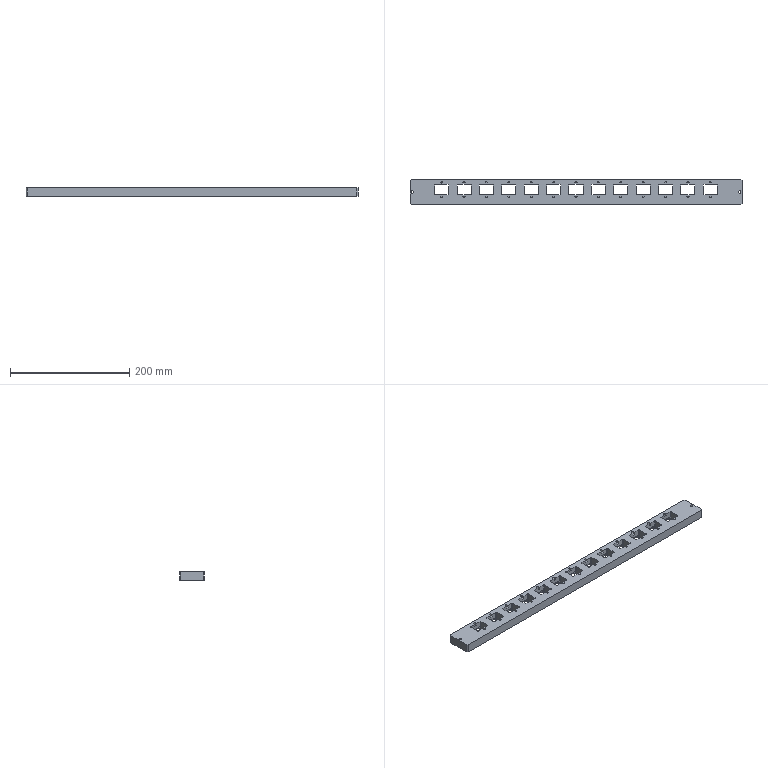NC program | NX | posted with a generic post | part box 556 x 41 x 15 mm
Lines 1 to 1304 of 144595:
N10 G17 G21 G94 G90
(ZLEVEL_PROFILE , TOOL : D10C)
N12 T10 M6
N14 G54
N16 G17 G0 G90 X-283.1 Y-3.442 S3500 M3
N18 G43 Z30. H10
N20 Z1.5
N22 G94 G1 Y18.82 Z0.333 F1000.
N24 X-282.978 Y19.653 Z0.289
N26 X-282.721 Y20.456 Z0.245
N28 X-282.336 Y21.205 Z0.201
N30 X-281.832 Y21.88 Z0.157
N32 X-279.38 Y24.332 Z-0.025
N34 X-278.705 Y24.836 Z-0.069
N36 X-277.956 Y25.221 Z-0.113
N38 X-277.153 Y25.478 Z-0.157
N40 X-276.32 Y25.6 Z-0.202
N42 X-276. Z-0.218
N44 X276. F2500.
N46 G2 X279.606 Y24.106 R5.1
N48 G1 X281.606 Y22.106
N50 G2 X283.1 Y18.5 R5.1
N52 G1 Y-18.5
N54 G2 X281.606 Y-22.106 R5.1
N56 G1 X279.606 Y-24.106
N58 G2 X276. Y-25.6 R5.1
N60 G1 X-276.
N62 G2 X-279.606 Y-24.106 R5.1
N64 G1 X-281.606 Y-22.106
N66 G2 X-283.1 Y-18.5 R5.1
N68 G1 Y18.5
N70 G2 X-281.606 Y22.106 R5.1
N72 G1 X-279.606 Y24.106
N74 G2 X-276. Y25.6 R5.1
N76 G1 X-263.489 Z-0.437
N78 X276.
N80 G2 X279.606 Y24.106 R5.1
N82 G1 X281.606 Y22.106
N84 G2 X283.1 Y18.5 R5.1
N86 G1 Y-18.5
N88 G2 X281.606 Y-22.106 R5.1
N90 G1 X279.606 Y-24.106
N92 G2 X276. Y-25.6 R5.1
N94 G1 X-276.
N96 G2 X-279.606 Y-24.106 R5.1
N98 G1 X-281.606 Y-22.106
N100 G2 X-283.1 Y-18.5 R5.1
N102 G1 Y18.5
N104 G2 X-281.606 Y22.106 R5.1
N106 G1 X-279.606 Y24.106
N108 G2 X-276. Y25.6 R5.1
N110 G1 X-263.489 Z-0.655
N112 X276.
N114 G2 X279.606 Y24.106 R5.1
N116 G1 X281.606 Y22.106
N118 G2 X283.1 Y18.5 R5.1
N120 G1 Y-18.5
N122 G2 X281.606 Y-22.106 R5.1
N124 G1 X279.606 Y-24.106
N126 G2 X276. Y-25.6 R5.1
N128 G1 X-276.
N130 G2 X-279.606 Y-24.106 R5.1
N132 G1 X-281.606 Y-22.106
N134 G2 X-283.1 Y-18.5 R5.1
N136 G1 Y18.5
N138 G2 X-281.606 Y22.106 R5.1
N140 G1 X-279.606 Y24.106
N142 G2 X-276. Y25.6 R5.1
N144 G1 X-263.489 Z-0.874
N146 X276.
N148 G2 X279.606 Y24.106 R5.1
N150 G1 X281.606 Y22.106
N152 G2 X283.1 Y18.5 R5.1
N154 G1 Y-18.5
N156 G2 X281.606 Y-22.106 R5.1
N158 G1 X279.606 Y-24.106
N160 G2 X276. Y-25.6 R5.1
N162 G1 X-276.
N164 G2 X-279.606 Y-24.106 R5.1
N166 G1 X-281.606 Y-22.106
N168 G2 X-283.1 Y-18.5 R5.1
N170 G1 Y18.5
N172 G2 X-281.606 Y22.106 R5.1
N174 G1 X-279.606 Y24.106
N176 G2 X-276. Y25.6 R5.1
N178 G1 X-263.489 Z-1.092
N180 X276.
N182 G2 X279.606 Y24.106 R5.1
N184 G1 X281.606 Y22.106
N186 G2 X283.1 Y18.5 R5.1
N188 G1 Y-18.5
N190 G2 X281.606 Y-22.106 R5.1
N192 G1 X279.606 Y-24.106
N194 G2 X276. Y-25.6 R5.1
N196 G1 X-276.
N198 G2 X-279.606 Y-24.106 R5.1
N200 G1 X-281.606 Y-22.106
N202 G2 X-283.1 Y-18.5 R5.1
N204 G1 Y18.5
N206 G2 X-281.606 Y22.106 R5.1
N208 G1 X-279.606 Y24.106
N210 G2 X-276. Y25.6 R5.1
N212 G1 X-263.489 Z-1.31
N214 X276.
N216 G2 X279.606 Y24.106 R5.1
N218 G1 X281.606 Y22.106
N220 G2 X283.1 Y18.5 R5.1
N222 G1 Y-18.5
N224 G2 X281.606 Y-22.106 R5.1
N226 G1 X279.606 Y-24.106
N228 G2 X276. Y-25.6 R5.1
N230 G1 X-276.
N232 G2 X-279.606 Y-24.106 R5.1
N234 G1 X-281.606 Y-22.106
N236 G2 X-283.1 Y-18.5 R5.1
N238 G1 Y18.5
N240 G2 X-281.606 Y22.106 R5.1
N242 G1 X-279.606 Y24.106
N244 G2 X-276. Y25.6 R5.1
N246 G1 X-263.489 Z-1.529
N248 X276.
N250 G2 X279.606 Y24.106 R5.1
N252 G1 X281.606 Y22.106
N254 G2 X283.1 Y18.5 R5.1
N256 G1 Y-18.5
N258 G2 X281.606 Y-22.106 R5.1
N260 G1 X279.606 Y-24.106
N262 G2 X276. Y-25.6 R5.1
N264 G1 X-276.
N266 G2 X-279.606 Y-24.106 R5.1
N268 G1 X-281.606 Y-22.106
N270 G2 X-283.1 Y-18.5 R5.1
N272 G1 Y18.5
N274 G2 X-281.606 Y22.106 R5.1
N276 G1 X-279.606 Y24.106
N278 G2 X-276. Y25.6 R5.1
N280 G1 X-263.489 Z-1.747
N282 X276.
N284 G2 X279.606 Y24.106 R5.1
N286 G1 X281.606 Y22.106
N288 G2 X283.1 Y18.5 R5.1
N290 G1 Y-18.5
N292 G2 X281.606 Y-22.106 R5.1
N294 G1 X279.606 Y-24.106
N296 G2 X276. Y-25.6 R5.1
N298 G1 X-276.
N300 G2 X-279.606 Y-24.106 R5.1
N302 G1 X-281.606 Y-22.106
N304 G2 X-283.1 Y-18.5 R5.1
N306 G1 Y18.5
N308 G2 X-281.606 Y22.106 R5.1
N310 G1 X-279.606 Y24.106
N312 G2 X-276. Y25.6 R5.1
N314 G1 X-263.489 Z-1.965
N316 X276.
N318 G2 X279.606 Y24.106 R5.1
N320 G1 X281.606 Y22.106
N322 G2 X283.1 Y18.5 R5.1
N324 G1 Y-18.5
N326 G2 X281.606 Y-22.106 R5.1
N328 G1 X279.606 Y-24.106
N330 G2 X276. Y-25.6 R5.1
N332 G1 X-276.
N334 G2 X-279.606 Y-24.106 R5.1
N336 G1 X-281.606 Y-22.106
N338 G2 X-283.1 Y-18.5 R5.1
N340 G1 Y18.5
N342 G2 X-281.606 Y22.106 R5.1
N344 G1 X-279.606 Y24.106
N346 G2 X-276. Y25.6 R5.1
N348 G1 X-263.489 Z-2.184
N350 X276.
N352 G2 X279.606 Y24.106 R5.1
N354 G1 X281.606 Y22.106
N356 G2 X283.1 Y18.5 R5.1
N358 G1 Y-18.5
N360 G2 X281.606 Y-22.106 R5.1
N362 G1 X279.606 Y-24.106
N364 G2 X276. Y-25.6 R5.1
N366 G1 X-276.
N368 G2 X-279.606 Y-24.106 R5.1
N370 G1 X-281.606 Y-22.106
N372 G2 X-283.1 Y-18.5 R5.1
N374 G1 Y18.5
N376 G2 X-281.606 Y22.106 R5.1
N378 G1 X-279.606 Y24.106
N380 G2 X-276. Y25.6 R5.1
N382 G1 X-263.489 Z-2.402
N384 X276.
N386 G2 X279.606 Y24.106 R5.1
N388 G1 X281.606 Y22.106
N390 G2 X283.1 Y18.5 R5.1
N392 G1 Y-18.5
N394 G2 X281.606 Y-22.106 R5.1
N396 G1 X279.606 Y-24.106
N398 G2 X276. Y-25.6 R5.1
N400 G1 X-276.
N402 G2 X-279.606 Y-24.106 R5.1
N404 G1 X-281.606 Y-22.106
N406 G2 X-283.1 Y-18.5 R5.1
N408 G1 Y18.5
N410 G2 X-281.606 Y22.106 R5.1
N412 G1 X-279.606 Y24.106
N414 G2 X-276. Y25.6 R5.1
N416 G1 X-263.489 Z-2.621
N418 X276.
N420 G2 X279.606 Y24.106 R5.1
N422 G1 X281.606 Y22.106
N424 G2 X283.1 Y18.5 R5.1
N426 G1 Y-18.5
N428 G2 X281.606 Y-22.106 R5.1
N430 G1 X279.606 Y-24.106
N432 G2 X276. Y-25.6 R5.1
N434 G1 X-276.
N436 G2 X-279.606 Y-24.106 R5.1
N438 G1 X-281.606 Y-22.106
N440 G2 X-283.1 Y-18.5 R5.1
N442 G1 Y18.5
N444 G2 X-281.606 Y22.106 R5.1
N446 G1 X-279.606 Y24.106
N448 G2 X-276. Y25.6 R5.1
N450 G1 X-263.489 Z-2.839
N452 X276.
N454 G2 X279.606 Y24.106 R5.1
N456 G1 X281.606 Y22.106
N458 G2 X283.1 Y18.5 R5.1
N460 G1 Y-18.5
N462 G2 X281.606 Y-22.106 R5.1
N464 G1 X279.606 Y-24.106
N466 G2 X276. Y-25.6 R5.1
N468 G1 X-276.
N470 G2 X-279.606 Y-24.106 R5.1
N472 G1 X-281.606 Y-22.106
N474 G2 X-283.1 Y-18.5 R5.1
N476 G1 Y18.5
N478 G2 X-281.606 Y22.106 R5.1
N480 G1 X-279.606 Y24.106
N482 G2 X-276. Y25.6 R5.1
N484 G1 X-263.489 Z-3.057
N486 X276.
N488 G2 X279.606 Y24.106 R5.1
N490 G1 X281.606 Y22.106
N492 G2 X283.1 Y18.5 R5.1
N494 G1 Y-18.5
N496 G2 X281.606 Y-22.106 R5.1
N498 G1 X279.606 Y-24.106
N500 G2 X276. Y-25.6 R5.1
N502 G1 X-276.
N504 G2 X-279.606 Y-24.106 R5.1
N506 G1 X-281.606 Y-22.106
N508 G2 X-283.1 Y-18.5 R5.1
N510 G1 Y18.5
N512 G2 X-281.606 Y22.106 R5.1
N514 G1 X-279.606 Y24.106
N516 G2 X-276. Y25.6 R5.1
N518 G1 X-263.489 Z-3.276
N520 X276.
N522 G2 X279.606 Y24.106 R5.1
N524 G1 X281.606 Y22.106
N526 G2 X283.1 Y18.5 R5.1
N528 G1 Y-18.5
N530 G2 X281.606 Y-22.106 R5.1
N532 G1 X279.606 Y-24.106
N534 G2 X276. Y-25.6 R5.1
N536 G1 X-276.
N538 G2 X-279.606 Y-24.106 R5.1
N540 G1 X-281.606 Y-22.106
N542 G2 X-283.1 Y-18.5 R5.1
N544 G1 Y18.5
N546 G2 X-281.606 Y22.106 R5.1
N548 G1 X-279.606 Y24.106
N550 G2 X-276. Y25.6 R5.1
N552 G1 X-263.489 Z-3.494
N554 X276.
N556 G2 X279.606 Y24.106 R5.1
N558 G1 X281.606 Y22.106
N560 G2 X283.1 Y18.5 R5.1
N562 G1 Y-18.5
N564 G2 X281.606 Y-22.106 R5.1
N566 G1 X279.606 Y-24.106
N568 G2 X276. Y-25.6 R5.1
N570 G1 X-276.
N572 G2 X-279.606 Y-24.106 R5.1
N574 G1 X-281.606 Y-22.106
N576 G2 X-283.1 Y-18.5 R5.1
N578 G1 Y18.5
N580 G2 X-281.606 Y22.106 R5.1
N582 G1 X-279.606 Y24.106
N584 G2 X-276. Y25.6 R5.1
N586 G1 X-263.489 Z-3.713
N588 X276.
N590 G2 X279.606 Y24.106 R5.1
N592 G1 X281.606 Y22.106
N594 G2 X283.1 Y18.5 R5.1
N596 G1 Y-18.5
N598 G2 X281.606 Y-22.106 R5.1
N600 G1 X279.606 Y-24.106
N602 G2 X276. Y-25.6 R5.1
N604 G1 X-276.
N606 G2 X-279.606 Y-24.106 R5.1
N608 G1 X-281.606 Y-22.106
N610 G2 X-283.1 Y-18.5 R5.1
N612 G1 Y18.5
N614 G2 X-281.606 Y22.106 R5.1
N616 G1 X-279.606 Y24.106
N618 G2 X-276. Y25.6 R5.1
N620 G1 X-263.489 Z-3.931
N622 X276.
N624 G2 X279.606 Y24.106 R5.1
N626 G1 X281.606 Y22.106
N628 G2 X283.1 Y18.5 R5.1
N630 G1 Y-18.5
N632 G2 X281.606 Y-22.106 R5.1
N634 G1 X279.606 Y-24.106
N636 G2 X276. Y-25.6 R5.1
N638 G1 X-276.
N640 G2 X-279.606 Y-24.106 R5.1
N642 G1 X-281.606 Y-22.106
N644 G2 X-283.1 Y-18.5 R5.1
N646 G1 Y18.5
N648 G2 X-281.606 Y22.106 R5.1
N650 G1 X-279.606 Y24.106
N652 G2 X-276. Y25.6 R5.1
N654 G1 X-263.489 Z-4.149
N656 X276.
N658 G2 X279.606 Y24.106 R5.1
N660 G1 X281.606 Y22.106
N662 G2 X283.1 Y18.5 R5.1
N664 G1 Y-18.5
N666 G2 X281.606 Y-22.106 R5.1
N668 G1 X279.606 Y-24.106
N670 G2 X276. Y-25.6 R5.1
N672 G1 X-276.
N674 G2 X-279.606 Y-24.106 R5.1
N676 G1 X-281.606 Y-22.106
N678 G2 X-283.1 Y-18.5 R5.1
N680 G1 Y18.5
N682 G2 X-281.606 Y22.106 R5.1
N684 G1 X-279.606 Y24.106
N686 G2 X-276. Y25.6 R5.1
N688 G1 X-263.489 Z-4.368
N690 X276.
N692 G2 X279.606 Y24.106 R5.1
N694 G1 X281.606 Y22.106
N696 G2 X283.1 Y18.5 R5.1
N698 G1 Y-18.5
N700 G2 X281.606 Y-22.106 R5.1
N702 G1 X279.606 Y-24.106
N704 G2 X276. Y-25.6 R5.1
N706 G1 X-276.
N708 G2 X-279.606 Y-24.106 R5.1
N710 G1 X-281.606 Y-22.106
N712 G2 X-283.1 Y-18.5 R5.1
N714 G1 Y18.5
N716 G2 X-281.606 Y22.106 R5.1
N718 G1 X-279.606 Y24.106
N720 G2 X-276. Y25.6 R5.1
N722 G1 X-263.489 Z-4.586
N724 X276.
N726 G2 X279.606 Y24.106 R5.1
N728 G1 X281.606 Y22.106
N730 G2 X283.1 Y18.5 R5.1
N732 G1 Y-18.5
N734 G2 X281.606 Y-22.106 R5.1
N736 G1 X279.606 Y-24.106
N738 G2 X276. Y-25.6 R5.1
N740 G1 X-276.
N742 G2 X-279.606 Y-24.106 R5.1
N744 G1 X-281.606 Y-22.106
N746 G2 X-283.1 Y-18.5 R5.1
N748 G1 Y18.5
N750 G2 X-281.606 Y22.106 R5.1
N752 G1 X-279.606 Y24.106
N754 G2 X-276. Y25.6 R5.1
N756 G1 X-263.489 Z-4.804
N758 X276.
N760 G2 X279.606 Y24.106 R5.1
N762 G1 X281.606 Y22.106
N764 G2 X283.1 Y18.5 R5.1
N766 G1 Y-18.5
N768 G2 X281.606 Y-22.106 R5.1
N770 G1 X279.606 Y-24.106
N772 G2 X276. Y-25.6 R5.1
N774 G1 X-276.
N776 G2 X-279.606 Y-24.106 R5.1
N778 G1 X-281.606 Y-22.106
N780 G2 X-283.1 Y-18.5 R5.1
N782 G1 Y18.5
N784 G2 X-281.606 Y22.106 R5.1
N786 G1 X-279.606 Y24.106
N788 G2 X-276. Y25.6 R5.1
N790 G1 X-263.489 Z-5.023
N792 X276.
N794 G2 X279.606 Y24.106 R5.1
N796 G1 X281.606 Y22.106
N798 G2 X283.1 Y18.5 R5.1
N800 G1 Y-18.5
N802 G2 X281.606 Y-22.106 R5.1
N804 G1 X279.606 Y-24.106
N806 G2 X276. Y-25.6 R5.1
N808 G1 X-276.
N810 G2 X-279.606 Y-24.106 R5.1
N812 G1 X-281.606 Y-22.106
N814 G2 X-283.1 Y-18.5 R5.1
N816 G1 Y18.5
N818 G2 X-281.606 Y22.106 R5.1
N820 G1 X-279.606 Y24.106
N822 G2 X-276. Y25.6 R5.1
N824 G1 X-263.489 Z-5.241
N826 X276.
N828 G2 X279.606 Y24.106 R5.1
N830 G1 X281.606 Y22.106
N832 G2 X283.1 Y18.5 R5.1
N834 G1 Y-18.5
N836 G2 X281.606 Y-22.106 R5.1
N838 G1 X279.606 Y-24.106
N840 G2 X276. Y-25.6 R5.1
N842 G1 X-276.
N844 G2 X-279.606 Y-24.106 R5.1
N846 G1 X-281.606 Y-22.106
N848 G2 X-283.1 Y-18.5 R5.1
N850 G1 Y18.5
N852 G2 X-281.606 Y22.106 R5.1
N854 G1 X-279.606 Y24.106
N856 G2 X-276. Y25.6 R5.1
N858 G1 X-263.489 Z-5.46
N860 X276.
N862 G2 X279.606 Y24.106 R5.1
N864 G1 X281.606 Y22.106
N866 G2 X283.1 Y18.5 R5.1
N868 G1 Y-18.5
N870 G2 X281.606 Y-22.106 R5.1
N872 G1 X279.606 Y-24.106
N874 G2 X276. Y-25.6 R5.1
N876 G1 X-276.
N878 G2 X-279.606 Y-24.106 R5.1
N880 G1 X-281.606 Y-22.106
N882 G2 X-283.1 Y-18.5 R5.1
N884 G1 Y18.5
N886 G2 X-281.606 Y22.106 R5.1
N888 G1 X-279.606 Y24.106
N890 G2 X-276. Y25.6 R5.1
N892 G1 X-263.489 Z-5.678
N894 X276.
N896 G2 X279.606 Y24.106 R5.1
N898 G1 X281.606 Y22.106
N900 G2 X283.1 Y18.5 R5.1
N902 G1 Y-18.5
N904 G2 X281.606 Y-22.106 R5.1
N906 G1 X279.606 Y-24.106
N908 G2 X276. Y-25.6 R5.1
N910 G1 X-276.
N912 G2 X-279.606 Y-24.106 R5.1
N914 G1 X-281.606 Y-22.106
N916 G2 X-283.1 Y-18.5 R5.1
N918 G1 Y18.5
N920 G2 X-281.606 Y22.106 R5.1
N922 G1 X-279.606 Y24.106
N924 G2 X-276. Y25.6 R5.1
N926 G1 X-263.489 Z-5.896
N928 X276.
N930 G2 X279.606 Y24.106 R5.1
N932 G1 X281.606 Y22.106
N934 G2 X283.1 Y18.5 R5.1
N936 G1 Y-18.5
N938 G2 X281.606 Y-22.106 R5.1
N940 G1 X279.606 Y-24.106
N942 G2 X276. Y-25.6 R5.1
N944 G1 X-276.
N946 G2 X-279.606 Y-24.106 R5.1
N948 G1 X-281.606 Y-22.106
N950 G2 X-283.1 Y-18.5 R5.1
N952 G1 Y18.5
N954 G2 X-281.606 Y22.106 R5.1
N956 G1 X-279.606 Y24.106
N958 G2 X-276. Y25.6 R5.1
N960 G1 X-263.489 Z-6.115
N962 X276.
N964 G2 X279.606 Y24.106 R5.1
N966 G1 X281.606 Y22.106
N968 G2 X283.1 Y18.5 R5.1
N970 G1 Y-18.5
N972 G2 X281.606 Y-22.106 R5.1
N974 G1 X279.606 Y-24.106
N976 G2 X276. Y-25.6 R5.1
N978 G1 X-276.
N980 G2 X-279.606 Y-24.106 R5.1
N982 G1 X-281.606 Y-22.106
N984 G2 X-283.1 Y-18.5 R5.1
N986 G1 Y18.5
N988 G2 X-281.606 Y22.106 R5.1
N990 G1 X-279.606 Y24.106
N992 G2 X-276. Y25.6 R5.1
N994 G1 X-263.489 Z-6.333
N996 X276.
N998 G2 X279.606 Y24.106 R5.1
N1000 G1 X281.606 Y22.106
N1002 G2 X283.1 Y18.5 R5.1
N1004 G1 Y-18.5
N1006 G2 X281.606 Y-22.106 R5.1
N1008 G1 X279.606 Y-24.106
N1010 G2 X276. Y-25.6 R5.1
N1012 G1 X-276.
N1014 G2 X-279.606 Y-24.106 R5.1
N1016 G1 X-281.606 Y-22.106
N1018 G2 X-283.1 Y-18.5 R5.1
N1020 G1 Y18.5
N1022 G2 X-281.606 Y22.106 R5.1
N1024 G1 X-279.606 Y24.106
N1026 G2 X-276. Y25.6 R5.1
N1028 G1 X-263.489 Z-6.551
N1030 X276.
N1032 G2 X279.606 Y24.106 R5.1
N1034 G1 X281.606 Y22.106
N1036 G2 X283.1 Y18.5 R5.1
N1038 G1 Y-18.5
N1040 G2 X281.606 Y-22.106 R5.1
N1042 G1 X279.606 Y-24.106
N1044 G2 X276. Y-25.6 R5.1
N1046 G1 X-276.
N1048 G2 X-279.606 Y-24.106 R5.1
N1050 G1 X-281.606 Y-22.106
N1052 G2 X-283.1 Y-18.5 R5.1
N1054 G1 Y18.5
N1056 G2 X-281.606 Y22.106 R5.1
N1058 G1 X-279.606 Y24.106
N1060 G2 X-276. Y25.6 R5.1
N1062 G1 X-263.489 Z-6.77
N1064 X276.
N1066 G2 X279.606 Y24.106 R5.1
N1068 G1 X281.606 Y22.106
N1070 G2 X283.1 Y18.5 R5.1
N1072 G1 Y-18.5
N1074 G2 X281.606 Y-22.106 R5.1
N1076 G1 X279.606 Y-24.106
N1078 G2 X276. Y-25.6 R5.1
N1080 G1 X-276.
N1082 G2 X-279.606 Y-24.106 R5.1
N1084 G1 X-281.606 Y-22.106
N1086 G2 X-283.1 Y-18.5 R5.1
N1088 G1 Y18.5
N1090 G2 X-281.606 Y22.106 R5.1
N1092 G1 X-279.606 Y24.106
N1094 G2 X-276. Y25.6 R5.1
N1096 G1 X-263.489 Z-6.988
N1098 X276.
N1100 G2 X279.606 Y24.106 R5.1
N1102 G1 X281.606 Y22.106
N1104 G2 X283.1 Y18.5 R5.1
N1106 G1 Y-18.5
N1108 G2 X281.606 Y-22.106 R5.1
N1110 G1 X279.606 Y-24.106
N1112 G2 X276. Y-25.6 R5.1
N1114 G1 X-276.
N1116 G2 X-279.606 Y-24.106 R5.1
N1118 G1 X-281.606 Y-22.106
N1120 G2 X-283.1 Y-18.5 R5.1
N1122 G1 Y18.5
N1124 G2 X-281.606 Y22.106 R5.1
N1126 G1 X-279.606 Y24.106
N1128 G2 X-276. Y25.6 R5.1
N1130 G1 X-263.489 Z-7.207
N1132 X276.
N1134 G2 X279.606 Y24.106 R5.1
N1136 G1 X281.606 Y22.106
N1138 G2 X283.1 Y18.5 R5.1
N1140 G1 Y-18.5
N1142 G2 X281.606 Y-22.106 R5.1
N1144 G1 X279.606 Y-24.106
N1146 G2 X276. Y-25.6 R5.1
N1148 G1 X-276.
N1150 G2 X-279.606 Y-24.106 R5.1
N1152 G1 X-281.606 Y-22.106
N1154 G2 X-283.1 Y-18.5 R5.1
N1156 G1 Y18.5
N1158 G2 X-281.606 Y22.106 R5.1
N1160 G1 X-279.606 Y24.106
N1162 G2 X-276. Y25.6 R5.1
N1164 G1 X-263.489 Z-7.425
N1166 X276.
N1168 G2 X279.606 Y24.106 R5.1
N1170 G1 X281.606 Y22.106
N1172 G2 X283.1 Y18.5 R5.1
N1174 G1 Y-18.5
N1176 G2 X281.606 Y-22.106 R5.1
N1178 G1 X279.606 Y-24.106
N1180 G2 X276. Y-25.6 R5.1
N1182 G1 X-276.
N1184 G2 X-279.606 Y-24.106 R5.1
N1186 G1 X-281.606 Y-22.106
N1188 G2 X-283.1 Y-18.5 R5.1
N1190 G1 Y18.5
N1192 G2 X-281.606 Y22.106 R5.1
N1194 G1 X-279.606 Y24.106
N1196 G2 X-276. Y25.6 R5.1
N1198 G1 X-263.489 Z-7.643
N1200 X276.
N1202 G2 X279.606 Y24.106 R5.1
N1204 G1 X281.606 Y22.106
N1206 G2 X283.1 Y18.5 R5.1
N1208 G1 Y-18.5
N1210 G2 X281.606 Y-22.106 R5.1
N1212 G1 X279.606 Y-24.106
N1214 G2 X276. Y-25.6 R5.1
N1216 G1 X-276.
N1218 G2 X-279.606 Y-24.106 R5.1
N1220 G1 X-281.606 Y-22.106
N1222 G2 X-283.1 Y-18.5 R5.1
N1224 G1 Y18.5
N1226 G2 X-281.606 Y22.106 R5.1
N1228 G1 X-279.606 Y24.106
N1230 G2 X-276. Y25.6 R5.1
N1232 G1 X-263.489 Z-7.862
N1234 X276.
N1236 G2 X279.606 Y24.106 R5.1
N1238 G1 X281.606 Y22.106
N1240 G2 X283.1 Y18.5 R5.1
N1242 G1 Y-18.5
N1244 G2 X281.606 Y-22.106 R5.1
N1246 G1 X279.606 Y-24.106
N1248 G2 X276. Y-25.6 R5.1
N1250 G1 X-276.
N1252 G2 X-279.606 Y-24.106 R5.1
N1254 G1 X-281.606 Y-22.106
N1256 G2 X-283.1 Y-18.5 R5.1
N1258 G1 Y18.5
N1260 G2 X-281.606 Y22.106 R5.1
N1262 G1 X-279.606 Y24.106
N1264 G2 X-276. Y25.6 R5.1
N1266 G1 X-263.489 Z-8.08
N1268 X276.
N1270 G2 X279.606 Y24.106 R5.1
N1272 G1 X281.606 Y22.106
N1274 G2 X283.1 Y18.5 R5.1
N1276 G1 Y-18.5
N1278 G2 X281.606 Y-22.106 R5.1
N1280 G1 X279.606 Y-24.106
N1282 G2 X276. Y-25.6 R5.1
N1284 G1 X-276.
N1286 G2 X-279.606 Y-24.106 R5.1
N1288 G1 X-281.606 Y-22.106
N1290 G2 X-283.1 Y-18.5 R5.1
N1292 G1 Y18.5
N1294 G2 X-281.606 Y22.106 R5.1
N1296 G1 X-279.606 Y24.106
N1298 G2 X-276. Y25.6 R5.1
N1300 G1 X-263.489 Z-8.299
N1302 X276.
N1304 G2 X279.606 Y24.106 R5.1
N1306 G1 X281.606 Y22.106
N1308 G2 X283.1 Y18.5 R5.1
N1310 G1 Y-18.5
N1312 G2 X281.606 Y-22.106 R5.1
N1314 G1 X279.606 Y-24.106
N1316 G2 X276. Y-25.6 R5.1
N1318 G1 X-276.
N1320 G2 X-279.606 Y-24.106 R5.1
N1322 G1 X-281.606 Y-22.106
N1324 G2 X-283.1 Y-18.5 R5.1
N1326 G1 Y18.5
N1328 G2 X-281.606 Y22.106 R5.1
N1330 G1 X-279.606 Y24.106
N1332 G2 X-276. Y25.6 R5.1
N1334 G1 X-263.489 Z-8.517
N1336 X276.
N1338 G2 X279.606 Y24.106 R5.1
N1340 G1 X281.606 Y22.106
N1342 G2 X283.1 Y18.5 R5.1
N1344 G1 Y-18.5
N1346 G2 X281.606 Y-22.106 R5.1
N1348 G1 X279.606 Y-24.106
N1350 G2 X276. Y-25.6 R5.1
N1352 G1 X-276.
N1354 G2 X-279.606 Y-24.106 R5.1
N1356 G1 X-281.606 Y-22.106
N1358 G2 X-283.1 Y-18.5 R5.1
N1360 G1 Y18.5
N1362 G2 X-281.606 Y22.106 R5.1
N1364 G1 X-279.606 Y24.106
N1366 G2 X-276. Y25.6 R5.1
N1368 G1 X-263.489 Z-8.735
N1370 X276.
N1372 G2 X279.606 Y24.106 R5.1
N1374 G1 X281.606 Y22.106
N1376 G2 X283.1 Y18.5 R5.1
N1378 G1 Y-18.5
N1380 G2 X281.606 Y-22.106 R5.1
N1382 G1 X279.606 Y-24.106
N1384 G2 X276. Y-25.6 R5.1
N1386 G1 X-276.
N1388 G2 X-279.606 Y-24.106 R5.1
N1390 G1 X-281.606 Y-22.106
N1392 G2 X-283.1 Y-18.5 R5.1
N1394 G1 Y18.5
N1396 G2 X-281.606 Y22.106 R5.1
N1398 G1 X-279.606 Y24.106
N1400 G2 X-276. Y25.6 R5.1
N1402 G1 X-263.489 Z-8.954
N1404 X276.
N1406 G2 X279.606 Y24.106 R5.1
N1408 G1 X281.606 Y22.106
N1410 G2 X283.1 Y18.5 R5.1
N1412 G1 Y-18.5
N1414 G2 X281.606 Y-22.106 R5.1
N1416 G1 X279.606 Y-24.106
N1418 G2 X276. Y-25.6 R5.1
N1420 G1 X-276.
N1422 G2 X-279.606 Y-24.106 R5.1
N1424 G1 X-281.606 Y-22.106
N1426 G2 X-283.1 Y-18.5 R5.1
N1428 G1 Y18.5
N1430 G2 X-281.606 Y22.106 R5.1
N1432 G1 X-279.606 Y24.106
N1434 G2 X-276. Y25.6 R5.1
N1436 G1 X-263.489 Z-9.172
N1438 X276.
N1440 G2 X279.606 Y24.106 R5.1
N1442 G1 X281.606 Y22.106
N1444 G2 X283.1 Y18.5 R5.1
N1446 G1 Y-18.5
N1448 G2 X281.606 Y-22.106 R5.1
N1450 G1 X279.606 Y-24.106
N1452 G2 X276. Y-25.6 R5.1
N1454 G1 X-276.
N1456 G2 X-279.606 Y-24.106 R5.1
N1458 G1 X-281.606 Y-22.106
N1460 G2 X-283.1 Y-18.5 R5.1
N1462 G1 Y18.5
N1464 G2 X-281.606 Y22.106 R5.1
N1466 G1 X-279.606 Y24.106
N1468 G2 X-276. Y25.6 R5.1
N1470 G1 X-263.489 Z-9.39
N1472 X276.
N1474 G2 X279.606 Y24.106 R5.1
N1476 G1 X281.606 Y22.106
N1478 G2 X283.1 Y18.5 R5.1
N1480 G1 Y-18.5
N1482 G2 X281.606 Y-22.106 R5.1
N1484 G1 X279.606 Y-24.106
N1486 G2 X276. Y-25.6 R5.1
N1488 G1 X-276.
N1490 G2 X-279.606 Y-24.106 R5.1
N1492 G1 X-281.606 Y-22.106
N1494 G2 X-283.1 Y-18.5 R5.1
N1496 G1 Y18.5
N1498 G2 X-281.606 Y22.106 R5.1
N1500 G1 X-279.606 Y24.106
N1502 G2 X-276. Y25.6 R5.1
N1504 G1 X-263.489 Z-9.609
N1506 X276.
N1508 G2 X279.606 Y24.106 R5.1
N1510 G1 X281.606 Y22.106
N1512 G2 X283.1 Y18.5 R5.1
N1514 G1 Y-18.5
N1516 G2 X281.606 Y-22.106 R5.1
N1518 G1 X279.606 Y-24.106
N1520 G2 X276. Y-25.6 R5.1
N1522 G1 X-276.
N1524 G2 X-279.606 Y-24.106 R5.1
N1526 G1 X-281.606 Y-22.106
N1528 G2 X-283.1 Y-18.5 R5.1
N1530 G1 Y18.5
N1532 G2 X-281.606 Y22.106 R5.1
N1534 G1 X-279.606 Y24.106
N1536 G2 X-276. Y25.6 R5.1
N1538 G1 X-263.489 Z-9.827
N1540 X276.
N1542 G2 X279.606 Y24.106 R5.1
N1544 G1 X281.606 Y22.106
N1546 G2 X283.1 Y18.5 R5.1
N1548 G1 Y-18.5
N1550 G2 X281.606 Y-22.106 R5.1
N1552 G1 X279.606 Y-24.106
N1554 G2 X276. Y-25.6 R5.1
N1556 G1 X-276.
N1558 G2 X-279.606 Y-24.106 R5.1
N1560 G1 X-281.606 Y-22.106
N1562 G2 X-283.1 Y-18.5 R5.1
N1564 G1 Y18.5
N1566 G2 X-281.606 Y22.106 R5.1
N1568 G1 X-279.606 Y24.106
N1570 G2 X-276. Y25.6 R5.1
N1572 G1 X-263.489 Z-10.046
N1574 X276.
N1576 G2 X279.606 Y24.106 R5.1
N1578 G1 X281.606 Y22.106
N1580 G2 X283.1 Y18.5 R5.1
N1582 G1 Y-18.5
N1584 G2 X281.606 Y-22.106 R5.1
N1586 G1 X279.606 Y-24.106
N1588 G2 X276. Y-25.6 R5.1
N1590 G1 X-276.
N1592 G2 X-279.606 Y-24.106 R5.1
N1594 G1 X-281.606 Y-22.106
N1596 G2 X-283.1 Y-18.5 R5.1
N1598 G1 Y18.5
N1600 G2 X-281.606 Y22.106 R5.1
N1602 G1 X-279.606 Y24.106
N1604 G2 X-276. Y25.6 R5.1
N1606 G1 X-263.489 Z-10.264
N1608 X276.
N1610 G2 X279.606 Y24.106 R5.1
N1612 G1 X281.606 Y22.106
N1614 G2 X283.1 Y18.5 R5.1
N1616 G1 Y-18.5
N1618 G2 X281.606 Y-22.106 R5.1
N1620 G1 X279.606 Y-24.106
N1622 G2 X276. Y-25.6 R5.1
N1624 G1 X-276.
N1626 G2 X-279.606 Y-24.106 R5.1
N1628 G1 X-281.606 Y-22.106
N1630 G2 X-283.1 Y-18.5 R5.1
N1632 G1 Y18.5
N1634 G2 X-281.606 Y22.106 R5.1
N1636 G1 X-279.606 Y24.106
N1638 G2 X-276. Y25.6 R5.1
N1640 G1 X-263.489 Z-10.482
N1642 X276.
N1644 G2 X279.606 Y24.106 R5.1
N1646 G1 X281.606 Y22.106
N1648 G2 X283.1 Y18.5 R5.1
N1650 G1 Y-18.5
N1652 G2 X281.606 Y-22.106 R5.1
N1654 G1 X279.606 Y-24.106
N1656 G2 X276. Y-25.6 R5.1
N1658 G1 X-276.
N1660 G2 X-279.606 Y-24.106 R5.1
N1662 G1 X-281.606 Y-22.106
N1664 G2 X-283.1 Y-18.5 R5.1
N1666 G1 Y18.5
N1668 G2 X-281.606 Y22.106 R5.1
N1670 G1 X-279.606 Y24.106
N1672 G2 X-276. Y25.6 R5.1
N1674 G1 X-263.489 Z-10.701
N1676 X276.
N1678 G2 X279.606 Y24.106 R5.1
N1680 G1 X281.606 Y22.106
N1682 G2 X283.1 Y18.5 R5.1
N1684 G1 Y-18.5
N1686 G2 X281.606 Y-22.106 R5.1
N1688 G1 X279.606 Y-24.106
N1690 G2 X276. Y-25.6 R5.1
N1692 G1 X-276.
N1694 G2 X-279.606 Y-24.106 R5.1
N1696 G1 X-281.606 Y-22.106
N1698 G2 X-283.1 Y-18.5 R5.1
N1700 G1 Y18.5
N1702 G2 X-281.606 Y22.106 R5.1
N1704 G1 X-279.606 Y24.106
N1706 G2 X-276. Y25.6 R5.1
N1708 G1 X-263.489 Z-10.919
N1710 X276.
N1712 G2 X279.606 Y24.106 R5.1
N1714 G1 X281.606 Y22.106
N1716 G2 X283.1 Y18.5 R5.1
N1718 G1 Y-18.5
N1720 G2 X281.606 Y-22.106 R5.1
N1722 G1 X279.606 Y-24.106
N1724 G2 X276. Y-25.6 R5.1
N1726 G1 X-276.
N1728 G2 X-279.606 Y-24.106 R5.1
N1730 G1 X-281.606 Y-22.106
N1732 G2 X-283.1 Y-18.5 R5.1
N1734 G1 Y18.5
N1736 G2 X-281.606 Y22.106 R5.1
N1738 G1 X-279.606 Y24.106
N1740 G2 X-276. Y25.6 R5.1
N1742 G1 X-263.489 Z-11.138
N1744 X276.
N1746 G2 X279.606 Y24.106 R5.1
N1748 G1 X281.606 Y22.106
N1750 G2 X283.1 Y18.5 R5.1
N1752 G1 Y-18.5
N1754 G2 X281.606 Y-22.106 R5.1
N1756 G1 X279.606 Y-24.106
N1758 G2 X276. Y-25.6 R5.1
N1760 G1 X-276.
N1762 G2 X-279.606 Y-24.106 R5.1
N1764 G1 X-281.606 Y-22.106
N1766 G2 X-283.1 Y-18.5 R5.1
N1768 G1 Y18.5
N1770 G2 X-281.606 Y22.106 R5.1
N1772 G1 X-279.606 Y24.106
N1774 G2 X-276. Y25.6 R5.1
N1776 G1 X-263.489 Z-11.356
N1778 X276.
N1780 G2 X279.606 Y24.106 R5.1
N1782 G1 X281.606 Y22.106
N1784 G2 X283.1 Y18.5 R5.1
N1786 G1 Y-18.5
N1788 G2 X281.606 Y-22.106 R5.1
N1790 G1 X279.606 Y-24.106
N1792 G2 X276. Y-25.6 R5.1
N1794 G1 X-276.
N1796 G2 X-279.606 Y-24.106 R5.1
N1798 G1 X-281.606 Y-22.106
N1800 G2 X-283.1 Y-18.5 R5.1
N1802 G1 Y18.5
N1804 G2 X-281.606 Y22.106 R5.1
N1806 G1 X-279.606 Y24.106
N1808 G2 X-276. Y25.6 R5.1
N1810 G1 X-263.489 Z-11.574
N1812 X276.
N1814 G2 X279.606 Y24.106 R5.1
N1816 G1 X281.606 Y22.106
N1818 G2 X283.1 Y18.5 R5.1
N1820 G1 Y-18.5
N1822 G2 X281.606 Y-22.106 R5.1
N1824 G1 X279.606 Y-24.106
N1826 G2 X276. Y-25.6 R5.1
N1828 G1 X-276.
N1830 G2 X-279.606 Y-24.106 R5.1
N1832 G1 X-281.606 Y-22.106
N1834 G2 X-283.1 Y-18.5 R5.1
N1836 G1 Y18.5
N1838 G2 X-281.606 Y22.106 R5.1
N1840 G1 X-279.606 Y24.106
N1842 G2 X-276. Y25.6 R5.1
N1844 G1 X-263.489 Z-11.793
N1846 X276.
N1848 G2 X279.606 Y24.106 R5.1
N1850 G1 X281.606 Y22.106
N1852 G2 X283.1 Y18.5 R5.1
N1854 G1 Y-18.5
N1856 G2 X281.606 Y-22.106 R5.1
N1858 G1 X279.606 Y-24.106
N1860 G2 X276. Y-25.6 R5.1
N1862 G1 X-276.
N1864 G2 X-279.606 Y-24.106 R5.1
N1866 G1 X-281.606 Y-22.106
N1868 G2 X-283.1 Y-18.5 R5.1
N1870 G1 Y18.5
N1872 G2 X-281.606 Y22.106 R5.1
N1874 G1 X-279.606 Y24.106
N1876 G2 X-276. Y25.6 R5.1
N1878 G1 X-263.489 Z-12.011
N1880 X276.
N1882 G2 X279.606 Y24.106 R5.1
N1884 G1 X281.606 Y22.106
N1886 G2 X283.1 Y18.5 R5.1
N1888 G1 Y-18.5
N1890 G2 X281.606 Y-22.106 R5.1
N1892 G1 X279.606 Y-24.106
N1894 G2 X276. Y-25.6 R5.1
N1896 G1 X-276.
N1898 G2 X-279.606 Y-24.106 R5.1
N1900 G1 X-281.606 Y-22.106
N1902 G2 X-283.1 Y-18.5 R5.1
N1904 G1 Y18.5
N1906 G2 X-281.606 Y22.106 R5.1
N1908 G1 X-279.606 Y24.106
N1910 G2 X-276. Y25.6 R5.1
N1912 G1 X-263.489 Z-12.229
N1914 X276.
N1916 G2 X279.606 Y24.106 R5.1
N1918 G1 X281.606 Y22.106
N1920 G2 X283.1 Y18.5 R5.1
N1922 G1 Y-18.5
N1924 G2 X281.606 Y-22.106 R5.1
N1926 G1 X279.606 Y-24.106
N1928 G2 X276. Y-25.6 R5.1
N1930 G1 X-276.
N1932 G2 X-279.606 Y-24.106 R5.1
N1934 G1 X-281.606 Y-22.106
N1936 G2 X-283.1 Y-18.5 R5.1
N1938 G1 Y18.5
N1940 G2 X-281.606 Y22.106 R5.1
N1942 G1 X-279.606 Y24.106
N1944 G2 X-276. Y25.6 R5.1
N1946 G1 X-263.489 Z-12.448
N1948 X276.
N1950 G2 X279.606 Y24.106 R5.1
N1952 G1 X281.606 Y22.106
N1954 G2 X283.1 Y18.5 R5.1
N1956 G1 Y-18.5
N1958 G2 X281.606 Y-22.106 R5.1
N1960 G1 X279.606 Y-24.106
N1962 G2 X276. Y-25.6 R5.1
N1964 G1 X-276.
N1966 G2 X-279.606 Y-24.106 R5.1
N1968 G1 X-281.606 Y-22.106
N1970 G2 X-283.1 Y-18.5 R5.1
N1972 G1 Y18.5
N1974 G2 X-281.606 Y22.106 R5.1
N1976 G1 X-279.606 Y24.106
N1978 G2 X-276. Y25.6 R5.1
N1980 G1 X-263.489 Z-12.666
N1982 X276.
N1984 G2 X279.606 Y24.106 R5.1
N1986 G1 X281.606 Y22.106
N1988 G2 X283.1 Y18.5 R5.1
N1990 G1 Y-18.5
N1992 G2 X281.606 Y-22.106 R5.1
N1994 G1 X279.606 Y-24.106
N1996 G2 X276. Y-25.6 R5.1
N1998 G1 X-276.
N2000 G2 X-279.606 Y-24.106 R5.1
N2002 G1 X-281.606 Y-22.106
N2004 G2 X-283.1 Y-18.5 R5.1
N2006 G1 Y18.5
N2008 G2 X-281.606 Y22.106 R5.1
N2010 G1 X-279.606 Y24.106
N2012 G2 X-276. Y25.6 R5.1
N2014 G1 X-263.489 Z-12.885
N2016 X276.
N2018 G2 X279.606 Y24.106 R5.1
N2020 G1 X281.606 Y22.106
N2022 G2 X283.1 Y18.5 R5.1
N2024 G1 Y-18.5
N2026 G2 X281.606 Y-22.106 R5.1
N2028 G1 X279.606 Y-24.106
N2030 G2 X276. Y-25.6 R5.1
N2032 G1 X-276.
N2034 G2 X-279.606 Y-24.106 R5.1
N2036 G1 X-281.606 Y-22.106
N2038 G2 X-283.1 Y-18.5 R5.1
N2040 G1 Y18.5
N2042 G2 X-281.606 Y22.106 R5.1
N2044 G1 X-279.606 Y24.106
N2046 G2 X-276. Y25.6 R5.1
N2048 G1 X-263.489 Z-13.103
N2050 X276.
N2052 G2 X279.606 Y24.106 R5.1
N2054 G1 X281.606 Y22.106
N2056 G2 X283.1 Y18.5 R5.1
N2058 G1 Y-18.5
N2060 G2 X281.606 Y-22.106 R5.1
N2062 G1 X279.606 Y-24.106
N2064 G2 X276. Y-25.6 R5.1
N2066 G1 X-276.
N2068 G2 X-279.606 Y-24.106 R5.1
N2070 G1 X-281.606 Y-22.106
N2072 G2 X-283.1 Y-18.5 R5.1
N2074 G1 Y18.5
N2076 G2 X-281.606 Y22.106 R5.1
N2078 G1 X-279.606 Y24.106
N2080 G2 X-276. Y25.6 R5.1
N2082 G1 X-263.489 Z-13.321
N2084 X276.
N2086 G2 X279.606 Y24.106 R5.1
N2088 G1 X281.606 Y22.106
N2090 G2 X283.1 Y18.5 R5.1
N2092 G1 Y-18.5
N2094 G2 X281.606 Y-22.106 R5.1
N2096 G1 X279.606 Y-24.106
N2098 G2 X276. Y-25.6 R5.1
N2100 G1 X-276.
N2102 G2 X-279.606 Y-24.106 R5.1
N2104 G1 X-281.606 Y-22.106
N2106 G2 X-283.1 Y-18.5 R5.1
N2108 G1 Y18.5
N2110 G2 X-281.606 Y22.106 R5.1
N2112 G1 X-279.606 Y24.106
N2114 G2 X-276. Y25.6 R5.1
N2116 G1 X-263.489 Z-13.54
N2118 X276.
N2120 G2 X279.606 Y24.106 R5.1
N2122 G1 X281.606 Y22.106
N2124 G2 X283.1 Y18.5 R5.1
N2126 G1 Y-18.5
N2128 G2 X281.606 Y-22.106 R5.1
N2130 G1 X279.606 Y-24.106
N2132 G2 X276. Y-25.6 R5.1
N2134 G1 X-276.
N2136 G2 X-279.606 Y-24.106 R5.1
N2138 G1 X-281.606 Y-22.106
N2140 G2 X-283.1 Y-18.5 R5.1
N2142 G1 Y18.5
N2144 G2 X-281.606 Y22.106 R5.1
N2146 G1 X-279.606 Y24.106
N2148 G2 X-276. Y25.6 R5.1
N2150 G1 X-263.489 Z-13.758
N2152 X276.
N2154 G2 X279.606 Y24.106 R5.1
N2156 G1 X281.606 Y22.106
N2158 G2 X283.1 Y18.5 R5.1
N2160 G1 Y-18.5
N2162 G2 X281.606 Y-22.106 R5.1
N2164 G1 X279.606 Y-24.106
N2166 G2 X276. Y-25.6 R5.1
N2168 G1 X-276.
N2170 G2 X-279.606 Y-24.106 R5.1
N2172 G1 X-281.606 Y-22.106
N2174 G2 X-283.1 Y-18.5 R5.1
N2176 G1 Y18.5
N2178 G2 X-281.606 Y22.106 R5.1
N2180 G1 X-279.606 Y24.106
N2182 G2 X-276. Y25.6 R5.1
N2184 G1 X-263.489 Z-13.976
N2186 X276.
N2188 G2 X279.606 Y24.106 R5.1
N2190 G1 X281.606 Y22.106
N2192 G2 X283.1 Y18.5 R5.1
N2194 G1 Y-18.5
N2196 G2 X281.606 Y-22.106 R5.1
N2198 G1 X279.606 Y-24.106
N2200 G2 X276. Y-25.6 R5.1
N2202 G1 X-276.
N2204 G2 X-279.606 Y-24.106 R5.1
N2206 G1 X-281.606 Y-22.106
N2208 G2 X-283.1 Y-18.5 R5.1
N2210 G1 Y18.5
N2212 G2 X-281.606 Y22.106 R5.1
N2214 G1 X-279.606 Y24.106
N2216 G2 X-276. Y25.6 R5.1
N2218 G1 X-263.489 Z-14.195
N2220 X276.
N2222 G2 X279.606 Y24.106 R5.1
N2224 G1 X281.606 Y22.106
N2226 G2 X283.1 Y18.5 R5.1
N2228 G1 Y-18.5
N2230 G2 X281.606 Y-22.106 R5.1
N2232 G1 X279.606 Y-24.106
N2234 G2 X276. Y-25.6 R5.1
N2236 G1 X-276.
N2238 G2 X-279.606 Y-24.106 R5.1
N2240 G1 X-281.606 Y-22.106
N2242 G2 X-283.1 Y-18.5 R5.1
N2244 G1 Y18.5
N2246 G2 X-281.606 Y22.106 R5.1
N2248 G1 X-279.606 Y24.106
N2250 G2 X-276. Y25.6 R5.1
N2252 G1 X-263.489 Z-14.413
N2254 X276.
N2256 G2 X279.606 Y24.106 R5.1
N2258 G1 X281.606 Y22.106
N2260 G2 X283.1 Y18.5 R5.1
N2262 G1 Y-18.5
N2264 G2 X281.606 Y-22.106 R5.1
N2266 G1 X279.606 Y-24.106
N2268 G2 X276. Y-25.6 R5.1
N2270 G1 X-276.
N2272 G2 X-279.606 Y-24.106 R5.1
N2274 G1 X-281.606 Y-22.106
N2276 G2 X-283.1 Y-18.5 R5.1
N2278 G1 Y18.5
N2280 G2 X-281.606 Y22.106 R5.1
N2282 G1 X-279.606 Y24.106
N2284 G2 X-276. Y25.6 R5.1
N2286 G1 X-263.489 Z-14.632
N2288 X276.
N2290 G2 X279.606 Y24.106 R5.1
N2292 G1 X281.606 Y22.106
N2294 G2 X283.1 Y18.5 R5.1
N2296 G1 Y-18.5
N2298 G2 X281.606 Y-22.106 R5.1
N2300 G1 X279.606 Y-24.106
N2302 G2 X276. Y-25.6 R5.1
N2304 G1 X-276.
N2306 G2 X-279.606 Y-24.106 R5.1
N2308 G1 X-281.606 Y-22.106
N2310 G2 X-283.1 Y-18.5 R5.1
N2312 G1 Y18.5
N2314 G2 X-281.606 Y22.106 R5.1
N2316 G1 X-279.606 Y24.106
N2318 G2 X-276. Y25.6 R5.1
N2320 G1 X-263.489 Z-14.85
N2322 X276.
N2324 G2 X279.606 Y24.106 R5.1
N2326 G1 X281.606 Y22.106
N2328 G2 X283.1 Y18.5 R5.1
N2330 G1 Y-18.5
N2332 G2 X281.606 Y-22.106 R5.1
N2334 G1 X279.606 Y-24.106
N2336 G2 X276. Y-25.6 R5.1
N2338 G1 X-276.
N2340 G2 X-279.606 Y-24.106 R5.1
N2342 G1 X-281.606 Y-22.106
N2344 G2 X-283.1 Y-18.5 R5.1
N2346 G1 Y18.5
N2348 G2 X-281.606 Y22.106 R5.1
N2350 G1 X-279.606 Y24.106
N2352 G2 X-276. Y25.6 R5.1
N2354 G1 X-263.489
N2356 Z-13.35
N2358 G0 Z30.
N2360 M5
(DRILLING , TOOL : ZXZ)
N2362 T01 M6
N2364 G54
N2366 G17 G0 G90 X-274. Y0. S3500 M3
N2368 G43 Z30. H1
N2370 G94 G81 G98 Z-1. F250. R3.
N2372 X274.
N2374 G80
N2376 G0 X274. Y0. Z30.
N2378 M5
(DRILLING_COPY , TOOL : 3.9ZT)
N2380 T09 M6
N2382 G54
N2384 G17 G0 G90 X-274. Y0. S2000 M3
N2386 G43 Z30. H9
N2388 G94 G83 G98 Z-14.85 F150. Q2. R3.
N2390 X274.
N2392 G80
N2394 G0 X274. Y0. Z30.
N2396 M5
(HOLE_MILLING , TOOL : D3)
N2398 T03 M6
N2400 G54
N2402 G17 G0 G90 X-274. Y0. S5000 M3
N2404 G43 Z30. H3
N2406 Z-13.
N2408 G94 G3 X-273.8 Y-0.2 R0.2 F1250.
N2410 X-273.6 Y0. R0.2
N2412 X-273.6 Y0. Z-13.06 I-0.4 J0.
N2414 X-273.6 Y0. Z-13.12 I-0.4 J0.
N2416 X-273.6 Y0. Z-13.18 I-0.4 J0.
N2418 X-273.6 Y0. Z-13.24 I-0.4 J0.
N2420 X-273.6 Y0. Z-13.3 I-0.4 J0.
N2422 X-273.6 Y0. Z-13.36 I-0.4 J0.
N2424 X-273.6 Y0. Z-13.42 I-0.4 J0.
N2426 X-273.6 Y0. Z-13.48 I-0.4 J0.
N2428 X-273.6 Y0. Z-13.54 I-0.4 J0.
N2430 X-273.6 Y0. Z-13.6 I-0.4 J0.
N2432 X-273.6 Y0. Z-13.66 I-0.4 J0.
N2434 X-273.6 Y0. Z-13.72 I-0.4 J0.
N2436 X-273.6 Y0. Z-13.78 I-0.4 J0.
N2438 X-273.6 Y0. Z-13.84 I-0.4 J0.
N2440 X-273.6 Y0. Z-13.9 I-0.4 J0.
N2442 X-273.6 Y0. Z-13.96 I-0.4 J0.
N2444 X-273.6 Y0. Z-14.02 I-0.4 J0.
N2446 X-273.6 Y0. Z-14.08 I-0.4 J0.
N2448 X-273.6 Y0. Z-14.14 I-0.4 J0.
N2450 X-273.6 Y0. Z-14.2 I-0.4 J0.
N2452 X-273.6 Y0. Z-14.26 I-0.4 J0.
N2454 X-273.6 Y0. Z-14.32 I-0.4 J0.
N2456 X-273.6 Y0. Z-14.38 I-0.4 J0.
N2458 X-273.6 Y0. Z-14.44 I-0.4 J0.
N2460 X-273.6 Y0. Z-14.5 I-0.4 J0.
N2462 X-273.6 Y0. Z-14.56 I-0.4 J0.
N2464 X-273.6 Y0. Z-14.62 I-0.4 J0.
N2466 X-273.6 Y0. Z-14.68 I-0.4 J0.
N2468 X-273.6 Y0. Z-14.74 I-0.4 J0.
N2470 X-273.6 Y0. Z-14.8 I-0.4 J0.
N2472 X-273.8 Y-0.346 Z-14.85 R-0.4
N2474 X-273.654 Y0.2 R0.4
N2476 X-273.8 Y-0.346 R-0.4
N2478 X-273.727 Y-0.073 R0.2
N2480 X-274. Y0. R0.2
N2482 G0 Z30.
N2484 X274.
N2486 Z-13.
N2488 G3 X274.2 Y-0.2 R0.2
N2490 X274.4 Y0. R0.2
N2492 X274.4 Y0. Z-13.06 I-0.4 J0.
N2494 X274.4 Y0. Z-13.12 I-0.4 J0.
N2496 X274.4 Y0. Z-13.18 I-0.4 J0.
N2498 X274.4 Y0. Z-13.24 I-0.4 J0.
N2500 X274.4 Y0. Z-13.3 I-0.4 J0.
N2502 X274.4 Y0. Z-13.36 I-0.4 J0.
N2504 X274.4 Y0. Z-13.42 I-0.4 J0.
N2506 X274.4 Y0. Z-13.48 I-0.4 J0.
N2508 X274.4 Y0. Z-13.54 I-0.4 J0.
N2510 X274.4 Y0. Z-13.6 I-0.4 J0.
N2512 X274.4 Y0. Z-13.66 I-0.4 J0.
N2514 X274.4 Y0. Z-13.72 I-0.4 J0.
N2516 X274.4 Y0. Z-13.78 I-0.4 J0.
N2518 X274.4 Y0. Z-13.84 I-0.4 J0.
N2520 X274.4 Y0. Z-13.9 I-0.4 J0.
N2522 X274.4 Y0. Z-13.96 I-0.4 J0.
N2524 X274.4 Y0. Z-14.02 I-0.4 J0.
N2526 X274.4 Y0. Z-14.08 I-0.4 J0.
N2528 X274.4 Y0. Z-14.14 I-0.4 J0.
N2530 X274.4 Y0. Z-14.2 I-0.4 J0.
N2532 X274.4 Y0. Z-14.26 I-0.4 J0.
N2534 X274.4 Y0. Z-14.32 I-0.4 J0.
N2536 X274.4 Y0. Z-14.38 I-0.4 J0.
N2538 X274.4 Y0. Z-14.44 I-0.4 J0.
N2540 X274.4 Y0. Z-14.5 I-0.4 J0.
N2542 X274.4 Y0. Z-14.56 I-0.4 J0.
N2544 X274.4 Y0. Z-14.62 I-0.4 J0.
N2546 X274.4 Y0. Z-14.68 I-0.4 J0.
N2548 X274.4 Y0. Z-14.74 I-0.4 J0.
N2550 X274.4 Y0. Z-14.8 I-0.4 J0.
N2552 X274.2 Y-0.346 Z-14.85 R-0.4
N2554 X274.346 Y0.2 R0.4
N2556 X274.2 Y-0.346 R-0.4
N2558 X274.273 Y-0.073 R0.2
N2560 X274. Y0. R0.2
N2562 G0 Z30.
N2564 M5
(DRILLING_COPY_COPY , TOOL : 4.0JD)
N2566 T08 M6
N2568 G54
N2570 G17 G0 G90 X-274. Y0. S1000 M3
N2572 G43 Z30. H8
N2574 G94 G85 G98 Z-14.85 F45. R3.
N2576 X274.
N2578 G80
N2580 G0 X274. Y0. Z30.
N2582 M5